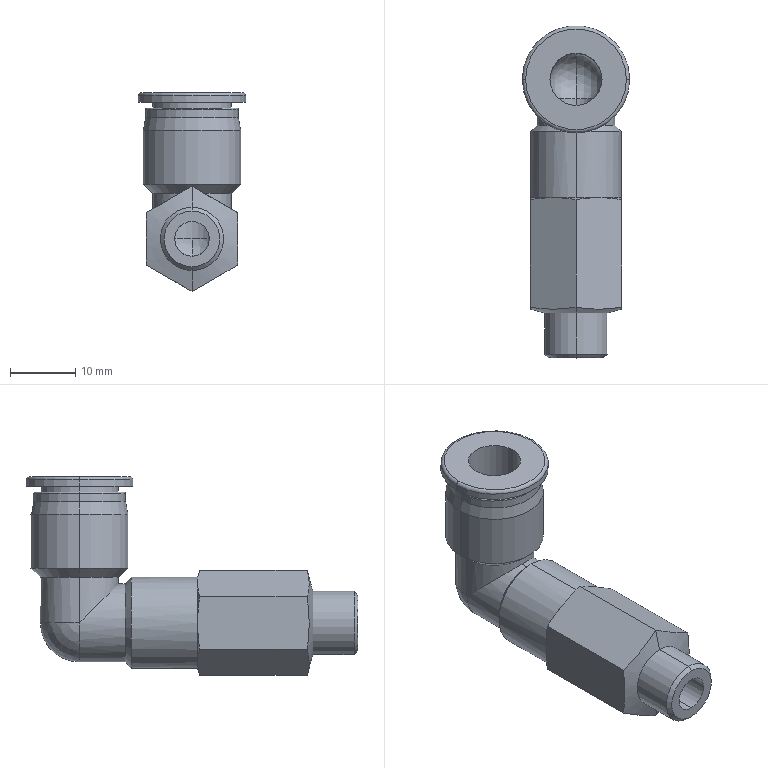Part | SolidWorks | features RevCut 2, Revolution 2, ICE 1 | 1 solid | 55 faces | box 16.5 x 51.05 x 30.583 mm | volume 7205 mm3 | cylinder 20 | cone 17 | plane 10 | torus 4 | sphere 4 | commonest cylinder face diameters 12 x6 5.333 x2 8 x2 9.728 x2 14 x2 14.25 x2